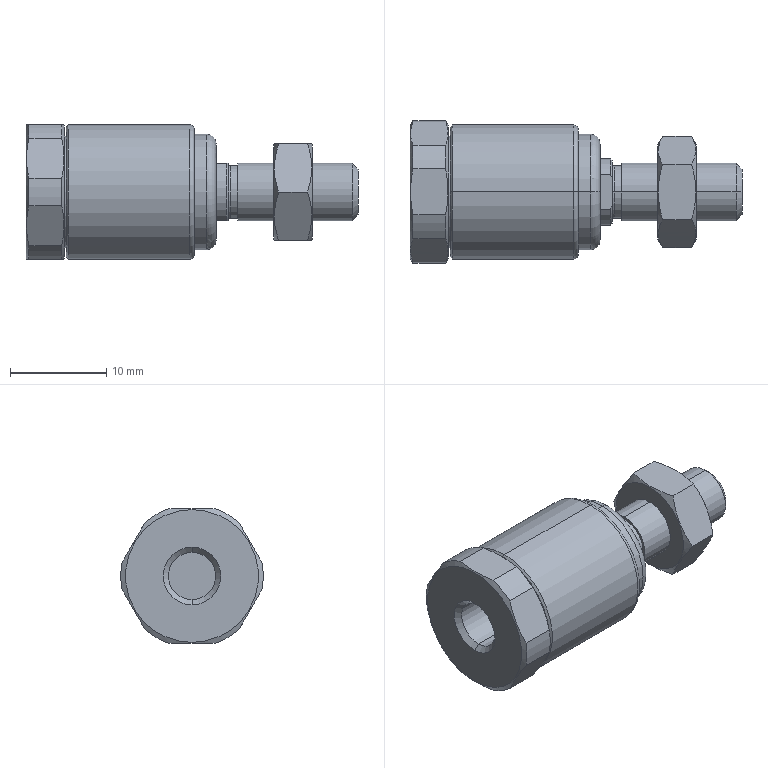Part | STEP file | 001-006-F-M6X100F | 1 solid | 75 faces | box 34.5 x 14.8 x 14 mm | volume 3454 mm3 | plane 27 | cylinder 22 | cone 18 | torus 8 | commonest cylinder face diameters 14.8 x6 6 x4 4.917 x2 5.5 x2 7 x2 11.6 x2